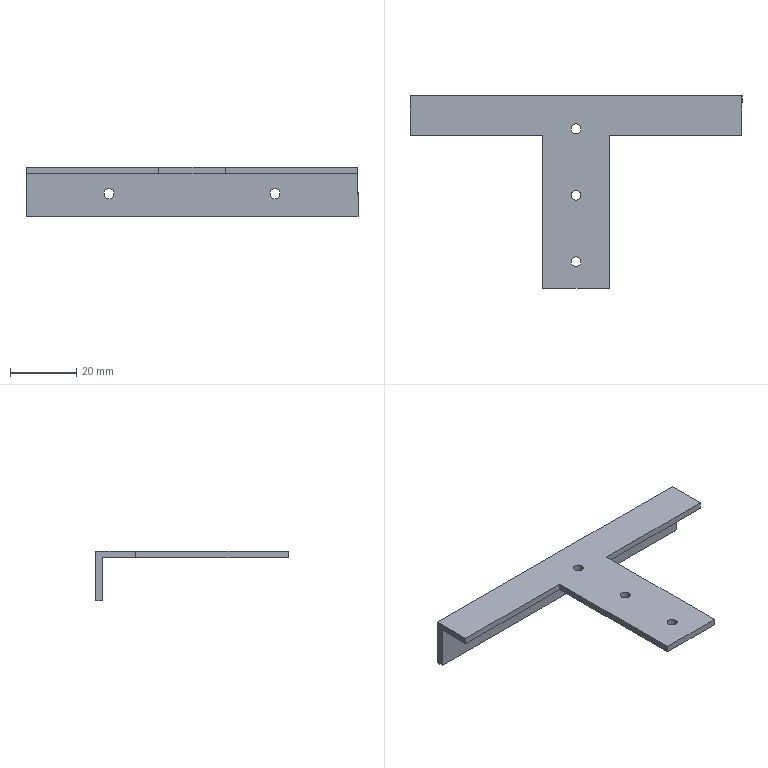Part | SolidWorks | features BaseBody 1 | 1 solid | 22 faces | box 100 x 58 x 15 mm | volume 6769 mm3 | plane 12 | cylinder 10 | commonest cylinder face diameters 3 x10
STEP:
#1=CARTESIAN_POINT('',(1.5,-30.,2.));
#2=VERTEX_POINT('',#1);
#3=CARTESIAN_POINT('',(-1.5,-30.,2.));
#4=VERTEX_POINT('',#3);
#5=CARTESIAN_POINT('',(0.,-30.,2.));
#6=DIRECTION('',(0.,0.,-1.));
#7=DIRECTION('',(-1.,0.,0.));
#8=AXIS2_PLACEMENT_3D('',#5,#6,#7);
#9=CIRCLE('',#8,1.5);
#10=EDGE_CURVE('',#2,#4,#9,.T.);
#11=ORIENTED_EDGE('',*,*,#10,.F.);
#12=CARTESIAN_POINT('',(1.5,-30.,0.));
#13=VERTEX_POINT('',#12);
#14=CARTESIAN_POINT('',(1.5,-30.,2.));
#15=DIRECTION('',(0.,0.,-1.));
#16=VECTOR('',#15,1000.);
#17=LINE('',#14,#16);
#18=EDGE_CURVE('',#2,#13,#17,.T.);
#19=ORIENTED_EDGE('',*,*,#18,.T.);
#20=CARTESIAN_POINT('',(-1.5,-30.,0.));
#21=VERTEX_POINT('',#20);
#22=CARTESIAN_POINT('',(0.,-30.,0.));
#23=DIRECTION('',(0.,0.,1.));
#24=DIRECTION('',(-1.,0.,0.));
#25=AXIS2_PLACEMENT_3D('',#22,#23,#24);
#26=CIRCLE('',#25,1.5);
#27=EDGE_CURVE('',#21,#13,#26,.T.);
#28=ORIENTED_EDGE('',*,*,#27,.F.);
#29=CARTESIAN_POINT('',(-1.5,-30.,2.));
#30=DIRECTION('',(0.,0.,-1.));
#31=VECTOR('',#30,1000.);
#32=LINE('',#29,#31);
#33=EDGE_CURVE('',#4,#21,#32,.T.);
#34=ORIENTED_EDGE('',*,*,#33,.F.);
#35=EDGE_LOOP('',(#11,#19,#28,#34));
#36=FACE_OUTER_BOUND('',#35,.T.);
#37=CARTESIAN_POINT('',(0.,-30.,2.));
#38=DIRECTION('',(0.,0.,-1.));
#39=DIRECTION('',(-1.,0.,0.));
#40=AXIS2_PLACEMENT_3D('',#37,#38,#39);
#41=CYLINDRICAL_SURFACE('',#40,1.5);
#42=ADVANCED_FACE('',(#36),#41,.F.);
#43=CARTESIAN_POINT('',(1.5,10.,2.));
#44=VERTEX_POINT('',#43);
#45=CARTESIAN_POINT('',(-1.5,10.,2.));
#46=VERTEX_POINT('',#45);
#47=CARTESIAN_POINT('',(0.,10.,2.));
#48=DIRECTION('',(0.,0.,-1.));
#49=DIRECTION('',(-1.,0.,0.));
#50=AXIS2_PLACEMENT_3D('',#47,#48,#49);
#51=CIRCLE('',#50,1.5);
#52=EDGE_CURVE('',#44,#46,#51,.T.);
#53=ORIENTED_EDGE('',*,*,#52,.F.);
#54=CARTESIAN_POINT('',(1.5,10.,0.));
#55=VERTEX_POINT('',#54);
#56=CARTESIAN_POINT('',(1.5,10.,2.));
#57=DIRECTION('',(0.,0.,-1.));
#58=VECTOR('',#57,1000.);
#59=LINE('',#56,#58);
#60=EDGE_CURVE('',#44,#55,#59,.T.);
#61=ORIENTED_EDGE('',*,*,#60,.T.);
#62=CARTESIAN_POINT('',(-1.5,10.,0.));
#63=VERTEX_POINT('',#62);
#64=CARTESIAN_POINT('',(0.,10.,0.));
#65=DIRECTION('',(0.,0.,1.));
#66=DIRECTION('',(-1.,0.,0.));
#67=AXIS2_PLACEMENT_3D('',#64,#65,#66);
#68=CIRCLE('',#67,1.5);
#69=EDGE_CURVE('',#63,#55,#68,.T.);
#70=ORIENTED_EDGE('',*,*,#69,.F.);
#71=CARTESIAN_POINT('',(-1.5,10.,2.));
#72=DIRECTION('',(0.,0.,-1.));
#73=VECTOR('',#72,1000.);
#74=LINE('',#71,#73);
#75=EDGE_CURVE('',#46,#63,#74,.T.);
#76=ORIENTED_EDGE('',*,*,#75,.F.);
#77=EDGE_LOOP('',(#53,#61,#70,#76));
#78=FACE_OUTER_BOUND('',#77,.T.);
#79=CARTESIAN_POINT('',(0.,10.,2.));
#80=DIRECTION('',(0.,0.,-1.));
#81=DIRECTION('',(-1.,0.,0.));
#82=AXIS2_PLACEMENT_3D('',#79,#80,#81);
#83=CYLINDRICAL_SURFACE('',#82,1.5);
#84=ADVANCED_FACE('',(#78),#83,.F.);
#85=CARTESIAN_POINT('',(1.5,-10.,2.));
#86=VERTEX_POINT('',#85);
#87=CARTESIAN_POINT('',(-1.5,-10.,2.));
#88=VERTEX_POINT('',#87);
#89=CARTESIAN_POINT('',(0.,-10.,2.));
#90=DIRECTION('',(0.,0.,-1.));
#91=DIRECTION('',(-1.,0.,0.));
#92=AXIS2_PLACEMENT_3D('',#89,#90,#91);
#93=CIRCLE('',#92,1.5);
#94=EDGE_CURVE('',#86,#88,#93,.T.);
#95=ORIENTED_EDGE('',*,*,#94,.F.);
#96=CARTESIAN_POINT('',(1.5,-10.,0.));
#97=VERTEX_POINT('',#96);
#98=CARTESIAN_POINT('',(1.5,-10.,2.));
#99=DIRECTION('',(0.,0.,-1.));
#100=VECTOR('',#99,1000.);
#101=LINE('',#98,#100);
#102=EDGE_CURVE('',#86,#97,#101,.T.);
#103=ORIENTED_EDGE('',*,*,#102,.T.);
#104=CARTESIAN_POINT('',(-1.5,-10.,0.));
#105=VERTEX_POINT('',#104);
#106=CARTESIAN_POINT('',(0.,-10.,0.));
#107=DIRECTION('',(0.,0.,1.));
#108=DIRECTION('',(-1.,0.,0.));
#109=AXIS2_PLACEMENT_3D('',#106,#107,#108);
#110=CIRCLE('',#109,1.5);
#111=EDGE_CURVE('',#105,#97,#110,.T.);
#112=ORIENTED_EDGE('',*,*,#111,.F.);
#113=CARTESIAN_POINT('',(-1.5,-10.,2.));
#114=DIRECTION('',(0.,0.,-1.));
#115=VECTOR('',#114,1000.);
#116=LINE('',#113,#115);
#117=EDGE_CURVE('',#88,#105,#116,.T.);
#118=ORIENTED_EDGE('',*,*,#117,.F.);
#119=EDGE_LOOP('',(#95,#103,#112,#118));
#120=FACE_OUTER_BOUND('',#119,.T.);
#121=CARTESIAN_POINT('',(0.,-10.,2.));
#122=DIRECTION('',(0.,0.,-1.));
#123=DIRECTION('',(-1.,0.,0.));
#124=AXIS2_PLACEMENT_3D('',#121,#122,#123);
#125=CYLINDRICAL_SURFACE('',#124,1.5);
#126=ADVANCED_FACE('',(#120),#125,.F.);
#127=CARTESIAN_POINT('',(25.,20.,-4.5));
#128=VERTEX_POINT('',#127);
#129=CARTESIAN_POINT('',(25.,20.,-7.5));
#130=VERTEX_POINT('',#129);
#131=CARTESIAN_POINT('',(25.,20.,-6.));
#132=DIRECTION('',(0.,-1.,0.));
#133=DIRECTION('',(0.,0.,-1.));
#134=AXIS2_PLACEMENT_3D('',#131,#132,#133);
#135=CIRCLE('',#134,1.5);
#136=EDGE_CURVE('',#128,#130,#135,.T.);
#137=ORIENTED_EDGE('',*,*,#136,.F.);
#138=CARTESIAN_POINT('',(25.,18.,-4.5));
#139=VERTEX_POINT('',#138);
#140=CARTESIAN_POINT('',(25.,28.,-4.5));
#141=DIRECTION('',(0.,-1.,0.));
#142=VECTOR('',#141,1000.);
#143=LINE('',#140,#142);
#144=EDGE_CURVE('',#128,#139,#143,.T.);
#145=ORIENTED_EDGE('',*,*,#144,.T.);
#146=CARTESIAN_POINT('',(25.,18.,-7.5));
#147=VERTEX_POINT('',#146);
#148=CARTESIAN_POINT('',(25.,18.,-6.));
#149=DIRECTION('',(0.,1.,0.));
#150=DIRECTION('',(0.,0.,-1.));
#151=AXIS2_PLACEMENT_3D('',#148,#149,#150);
#152=CIRCLE('',#151,1.5);
#153=EDGE_CURVE('',#147,#139,#152,.T.);
#154=ORIENTED_EDGE('',*,*,#153,.F.);
#155=CARTESIAN_POINT('',(25.,28.,-7.5));
#156=DIRECTION('',(0.,-1.,0.));
#157=VECTOR('',#156,1000.);
#158=LINE('',#155,#157);
#159=EDGE_CURVE('',#130,#147,#158,.T.);
#160=ORIENTED_EDGE('',*,*,#159,.F.);
#161=EDGE_LOOP('',(#137,#145,#154,#160));
#162=FACE_OUTER_BOUND('',#161,.T.);
#163=CARTESIAN_POINT('',(25.,28.,-6.));
#164=DIRECTION('',(0.,-1.,0.));
#165=DIRECTION('',(0.,0.,-1.));
#166=AXIS2_PLACEMENT_3D('',#163,#164,#165);
#167=CYLINDRICAL_SURFACE('',#166,1.5);
#168=ADVANCED_FACE('',(#162),#167,.F.);
#169=CARTESIAN_POINT('',(-25.,20.,-4.5));
#170=VERTEX_POINT('',#169);
#171=CARTESIAN_POINT('',(-25.,20.,-7.5));
#172=VERTEX_POINT('',#171);
#173=CARTESIAN_POINT('',(-25.,20.,-6.));
#174=DIRECTION('',(0.,-1.,0.));
#175=DIRECTION('',(0.,0.,-1.));
#176=AXIS2_PLACEMENT_3D('',#173,#174,#175);
#177=CIRCLE('',#176,1.5);
#178=EDGE_CURVE('',#170,#172,#177,.T.);
#179=ORIENTED_EDGE('',*,*,#178,.F.);
#180=CARTESIAN_POINT('',(-25.,18.,-4.5));
#181=VERTEX_POINT('',#180);
#182=CARTESIAN_POINT('',(-25.,28.,-4.5));
#183=DIRECTION('',(0.,-1.,0.));
#184=VECTOR('',#183,1000.);
#185=LINE('',#182,#184);
#186=EDGE_CURVE('',#170,#181,#185,.T.);
#187=ORIENTED_EDGE('',*,*,#186,.T.);
#188=CARTESIAN_POINT('',(-25.,18.,-7.5));
#189=VERTEX_POINT('',#188);
#190=CARTESIAN_POINT('',(-25.,18.,-6.));
#191=DIRECTION('',(0.,1.,0.));
#192=DIRECTION('',(0.,0.,-1.));
#193=AXIS2_PLACEMENT_3D('',#190,#191,#192);
#194=CIRCLE('',#193,1.5);
#195=EDGE_CURVE('',#189,#181,#194,.T.);
#196=ORIENTED_EDGE('',*,*,#195,.F.);
#197=CARTESIAN_POINT('',(-25.,28.,-7.5));
#198=DIRECTION('',(0.,-1.,0.));
#199=VECTOR('',#198,1000.);
#200=LINE('',#197,#199);
#201=EDGE_CURVE('',#172,#189,#200,.T.);
#202=ORIENTED_EDGE('',*,*,#201,.F.);
#203=EDGE_LOOP('',(#179,#187,#196,#202));
#204=FACE_OUTER_BOUND('',#203,.T.);
#205=CARTESIAN_POINT('',(-25.,28.,-6.));
#206=DIRECTION('',(0.,-1.,0.));
#207=DIRECTION('',(0.,0.,-1.));
#208=AXIS2_PLACEMENT_3D('',#205,#206,#207);
#209=CYLINDRICAL_SURFACE('',#208,1.5);
#210=ADVANCED_FACE('',(#204),#209,.F.);
#211=CARTESIAN_POINT('',(0.,-30.,2.));
#212=DIRECTION('',(0.,0.,-1.));
#213=DIRECTION('',(-1.,0.,0.));
#214=AXIS2_PLACEMENT_3D('',#211,#212,#213);
#215=CIRCLE('',#214,1.5);
#216=EDGE_CURVE('',#4,#2,#215,.T.);
#217=ORIENTED_EDGE('',*,*,#216,.T.);
#218=ORIENTED_EDGE('',*,*,#10,.T.);
#219=EDGE_LOOP('',(#217,#218));
#220=FACE_BOUND('',#219,.T.);
#221=CARTESIAN_POINT('',(0.,10.,2.));
#222=DIRECTION('',(0.,0.,-1.));
#223=DIRECTION('',(-1.,0.,0.));
#224=AXIS2_PLACEMENT_3D('',#221,#222,#223);
#225=CIRCLE('',#224,1.5);
#226=EDGE_CURVE('',#46,#44,#225,.T.);
#227=ORIENTED_EDGE('',*,*,#226,.T.);
#228=ORIENTED_EDGE('',*,*,#52,.T.);
#229=EDGE_LOOP('',(#227,#228));
#230=FACE_BOUND('',#229,.T.);
#231=CARTESIAN_POINT('',(50.,8.,2.));
#232=VERTEX_POINT('',#231);
#233=CARTESIAN_POINT('',(50.,20.,2.));
#234=VERTEX_POINT('',#233);
#235=CARTESIAN_POINT('',(50.,0.,2.));
#236=DIRECTION('',(0.,1.,0.));
#237=VECTOR('',#236,1000.);
#238=LINE('',#235,#237);
#239=EDGE_CURVE('',#232,#234,#238,.T.);
#240=ORIENTED_EDGE('',*,*,#239,.T.);
#241=CARTESIAN_POINT('',(-50.,20.,2.));
#242=VERTEX_POINT('',#241);
#243=CARTESIAN_POINT('',(0.,20.,2.));
#244=DIRECTION('',(-1.,0.,0.));
#245=VECTOR('',#244,1000.);
#246=LINE('',#243,#245);
#247=EDGE_CURVE('',#234,#242,#246,.T.);
#248=ORIENTED_EDGE('',*,*,#247,.T.);
#249=CARTESIAN_POINT('',(-50.,8.,2.));
#250=VERTEX_POINT('',#249);
#251=CARTESIAN_POINT('',(-50.,0.,2.));
#252=DIRECTION('',(0.,-1.,0.));
#253=VECTOR('',#252,1000.);
#254=LINE('',#251,#253);
#255=EDGE_CURVE('',#242,#250,#254,.T.);
#256=ORIENTED_EDGE('',*,*,#255,.T.);
#257=CARTESIAN_POINT('',(-10.,8.,2.));
#258=VERTEX_POINT('',#257);
#259=CARTESIAN_POINT('',(0.,8.,2.));
#260=DIRECTION('',(1.,0.,0.));
#261=VECTOR('',#260,1000.);
#262=LINE('',#259,#261);
#263=EDGE_CURVE('',#250,#258,#262,.T.);
#264=ORIENTED_EDGE('',*,*,#263,.T.);
#265=CARTESIAN_POINT('',(-10.,-38.,2.));
#266=VERTEX_POINT('',#265);
#267=CARTESIAN_POINT('',(-10.,0.,2.));
#268=DIRECTION('',(0.,-1.,0.));
#269=VECTOR('',#268,1000.);
#270=LINE('',#267,#269);
#271=EDGE_CURVE('',#258,#266,#270,.T.);
#272=ORIENTED_EDGE('',*,*,#271,.T.);
#273=CARTESIAN_POINT('',(10.,-38.,2.));
#274=VERTEX_POINT('',#273);
#275=CARTESIAN_POINT('',(0.,-38.,2.));
#276=DIRECTION('',(1.,0.,0.));
#277=VECTOR('',#276,1000.);
#278=LINE('',#275,#277);
#279=EDGE_CURVE('',#266,#274,#278,.T.);
#280=ORIENTED_EDGE('',*,*,#279,.T.);
#281=CARTESIAN_POINT('',(10.,8.,2.));
#282=VERTEX_POINT('',#281);
#283=CARTESIAN_POINT('',(10.,0.,2.));
#284=DIRECTION('',(0.,1.,0.));
#285=VECTOR('',#284,1000.);
#286=LINE('',#283,#285);
#287=EDGE_CURVE('',#274,#282,#286,.T.);
#288=ORIENTED_EDGE('',*,*,#287,.T.);
#289=CARTESIAN_POINT('',(0.,8.,2.));
#290=DIRECTION('',(1.,0.,0.));
#291=VECTOR('',#290,1000.);
#292=LINE('',#289,#291);
#293=EDGE_CURVE('',#282,#232,#292,.T.);
#294=ORIENTED_EDGE('',*,*,#293,.T.);
#295=EDGE_LOOP('',(#240,#248,#256,#264,#272,#280,#288,#294));
#296=FACE_OUTER_BOUND('',#295,.T.);
#297=CARTESIAN_POINT('',(0.,-10.,2.));
#298=DIRECTION('',(0.,0.,-1.));
#299=DIRECTION('',(-1.,0.,0.));
#300=AXIS2_PLACEMENT_3D('',#297,#298,#299);
#301=CIRCLE('',#300,1.5);
#302=EDGE_CURVE('',#88,#86,#301,.T.);
#303=ORIENTED_EDGE('',*,*,#302,.T.);
#304=ORIENTED_EDGE('',*,*,#94,.T.);
#305=EDGE_LOOP('',(#303,#304));
#306=FACE_BOUND('',#305,.T.);
#307=CARTESIAN_POINT('',(0.,0.,2.));
#308=DIRECTION('',(0.,0.,1.));
#309=DIRECTION('',(1.,0.,0.));
#310=AXIS2_PLACEMENT_3D('',#307,#308,#309);
#311=PLANE('',#310);
#312=ADVANCED_FACE('',(#220,#230,#296,#306),#311,.T.);
#313=ORIENTED_EDGE('',*,*,#18,.F.);
#314=ORIENTED_EDGE('',*,*,#216,.F.);
#315=ORIENTED_EDGE('',*,*,#33,.T.);
#316=CARTESIAN_POINT('',(0.,-30.,0.));
#317=DIRECTION('',(0.,0.,1.));
#318=DIRECTION('',(-1.,0.,0.));
#319=AXIS2_PLACEMENT_3D('',#316,#317,#318);
#320=CIRCLE('',#319,1.5);
#321=EDGE_CURVE('',#13,#21,#320,.T.);
#322=ORIENTED_EDGE('',*,*,#321,.F.);
#323=EDGE_LOOP('',(#313,#314,#315,#322));
#324=FACE_OUTER_BOUND('',#323,.T.);
#325=CARTESIAN_POINT('',(0.,-30.,2.));
#326=DIRECTION('',(0.,0.,-1.));
#327=DIRECTION('',(-1.,0.,0.));
#328=AXIS2_PLACEMENT_3D('',#325,#326,#327);
#329=CYLINDRICAL_SURFACE('',#328,1.5);
#330=ADVANCED_FACE('',(#324),#329,.F.);
#331=ORIENTED_EDGE('',*,*,#60,.F.);
#332=ORIENTED_EDGE('',*,*,#226,.F.);
#333=ORIENTED_EDGE('',*,*,#75,.T.);
#334=CARTESIAN_POINT('',(0.,10.,0.));
#335=DIRECTION('',(0.,0.,1.));
#336=DIRECTION('',(-1.,0.,0.));
#337=AXIS2_PLACEMENT_3D('',#334,#335,#336);
#338=CIRCLE('',#337,1.5);
#339=EDGE_CURVE('',#55,#63,#338,.T.);
#340=ORIENTED_EDGE('',*,*,#339,.F.);
#341=EDGE_LOOP('',(#331,#332,#333,#340));
#342=FACE_OUTER_BOUND('',#341,.T.);
#343=CARTESIAN_POINT('',(0.,10.,2.));
#344=DIRECTION('',(0.,0.,-1.));
#345=DIRECTION('',(-1.,0.,0.));
#346=AXIS2_PLACEMENT_3D('',#343,#344,#345);
#347=CYLINDRICAL_SURFACE('',#346,1.5);
#348=ADVANCED_FACE('',(#342),#347,.F.);
#349=CARTESIAN_POINT('',(25.,20.,-6.));
#350=DIRECTION('',(0.,-1.,0.));
#351=DIRECTION('',(0.,0.,-1.));
#352=AXIS2_PLACEMENT_3D('',#349,#350,#351);
#353=CIRCLE('',#352,1.5);
#354=EDGE_CURVE('',#130,#128,#353,.T.);
#355=ORIENTED_EDGE('',*,*,#354,.T.);
#356=ORIENTED_EDGE('',*,*,#136,.T.);
#357=EDGE_LOOP('',(#355,#356));
#358=FACE_BOUND('',#357,.T.);
#359=CARTESIAN_POINT('',(-25.,20.,-6.));
#360=DIRECTION('',(0.,-1.,0.));
#361=DIRECTION('',(0.,0.,-1.));
#362=AXIS2_PLACEMENT_3D('',#359,#360,#361);
#363=CIRCLE('',#362,1.5);
#364=EDGE_CURVE('',#172,#170,#363,.T.);
#365=ORIENTED_EDGE('',*,*,#364,.T.);
#366=ORIENTED_EDGE('',*,*,#178,.T.);
#367=EDGE_LOOP('',(#365,#366));
#368=FACE_BOUND('',#367,.T.);
#369=CARTESIAN_POINT('',(50.,20.,-13.));
#370=VERTEX_POINT('',#369);
#371=CARTESIAN_POINT('',(50.,20.,0.));
#372=DIRECTION('',(0.,0.,-1.));
#373=VECTOR('',#372,1000.);
#374=LINE('',#371,#373);
#375=EDGE_CURVE('',#234,#370,#374,.T.);
#376=ORIENTED_EDGE('',*,*,#375,.T.);
#377=CARTESIAN_POINT('',(-50.,20.,-13.));
#378=VERTEX_POINT('',#377);
#379=CARTESIAN_POINT('',(0.,20.,-13.));
#380=DIRECTION('',(-1.,0.,0.));
#381=VECTOR('',#380,1000.);
#382=LINE('',#379,#381);
#383=EDGE_CURVE('',#370,#378,#382,.T.);
#384=ORIENTED_EDGE('',*,*,#383,.T.);
#385=CARTESIAN_POINT('',(-50.,20.,0.));
#386=DIRECTION('',(0.,0.,1.));
#387=VECTOR('',#386,1000.);
#388=LINE('',#385,#387);
#389=EDGE_CURVE('',#378,#242,#388,.T.);
#390=ORIENTED_EDGE('',*,*,#389,.T.);
#391=ORIENTED_EDGE('',*,*,#247,.F.);
#392=EDGE_LOOP('',(#376,#384,#390,#391));
#393=FACE_OUTER_BOUND('',#392,.T.);
#394=CARTESIAN_POINT('',(0.,20.,0.));
#395=DIRECTION('',(0.,1.,0.));
#396=DIRECTION('',(0.,0.,1.));
#397=AXIS2_PLACEMENT_3D('',#394,#395,#396);
#398=PLANE('',#397);
#399=ADVANCED_FACE('',(#358,#368,#393),#398,.T.);
#400=CARTESIAN_POINT('',(50.,18.,-13.));
#401=VERTEX_POINT('',#400);
#402=CARTESIAN_POINT('',(50.,18.,0.));
#403=VERTEX_POINT('',#402);
#404=CARTESIAN_POINT('',(50.,18.,2.));
#405=DIRECTION('',(0.,0.,1.));
#406=VECTOR('',#405,1000.);
#407=LINE('',#404,#406);
#408=EDGE_CURVE('',#401,#403,#407,.T.);
#409=ORIENTED_EDGE('',*,*,#408,.F.);
#410=CARTESIAN_POINT('',(50.,18.,-13.));
#411=DIRECTION('',(0.,-1.,0.));
#412=VECTOR('',#411,1000.);
#413=LINE('',#410,#412);
#414=EDGE_CURVE('',#370,#401,#413,.T.);
#415=ORIENTED_EDGE('',*,*,#414,.F.);
#416=ORIENTED_EDGE('',*,*,#375,.F.);
#417=ORIENTED_EDGE('',*,*,#239,.F.);
#418=CARTESIAN_POINT('',(50.,8.,0.));
#419=VERTEX_POINT('',#418);
#420=CARTESIAN_POINT('',(50.,8.,2.));
#421=DIRECTION('',(0.,0.,1.));
#422=VECTOR('',#421,1000.);
#423=LINE('',#420,#422);
#424=EDGE_CURVE('',#419,#232,#423,.T.);
#425=ORIENTED_EDGE('',*,*,#424,.F.);
#426=CARTESIAN_POINT('',(50.,18.,0.));
#427=DIRECTION('',(0.,-1.,0.));
#428=VECTOR('',#427,1000.);
#429=LINE('',#426,#428);
#430=EDGE_CURVE('',#403,#419,#429,.T.);
#431=ORIENTED_EDGE('',*,*,#430,.F.);
#432=EDGE_LOOP('',(#409,#415,#416,#417,#425,#431));
#433=FACE_OUTER_BOUND('',#432,.T.);
#434=CARTESIAN_POINT('',(50.,18.,2.));
#435=DIRECTION('',(-1.,0.,0.));
#436=DIRECTION('',(0.,-1.,0.));
#437=AXIS2_PLACEMENT_3D('',#434,#435,#436);
#438=PLANE('',#437);
#439=ADVANCED_FACE('',(#433),#438,.F.);
#440=ORIENTED_EDGE('',*,*,#424,.T.);
#441=ORIENTED_EDGE('',*,*,#293,.F.);
#442=CARTESIAN_POINT('',(10.,8.,0.));
#443=VERTEX_POINT('',#442);
#444=CARTESIAN_POINT('',(10.,8.,2.));
#445=DIRECTION('',(0.,0.,1.));
#446=VECTOR('',#445,1000.);
#447=LINE('',#444,#446);
#448=EDGE_CURVE('',#443,#282,#447,.T.);
#449=ORIENTED_EDGE('',*,*,#448,.F.);
#450=CARTESIAN_POINT('',(50.,8.,0.));
#451=DIRECTION('',(-1.,0.,0.));
#452=VECTOR('',#451,1000.);
#453=LINE('',#450,#452);
#454=EDGE_CURVE('',#419,#443,#453,.T.);
#455=ORIENTED_EDGE('',*,*,#454,.F.);
#456=EDGE_LOOP('',(#440,#441,#449,#455));
#457=FACE_OUTER_BOUND('',#456,.T.);
#458=CARTESIAN_POINT('',(50.,8.,2.));
#459=DIRECTION('',(0.,1.,0.));
#460=DIRECTION('',(-1.,0.,0.));
#461=AXIS2_PLACEMENT_3D('',#458,#459,#460);
#462=PLANE('',#461);
#463=ADVANCED_FACE('',(#457),#462,.F.);
#464=ORIENTED_EDGE('',*,*,#448,.T.);
#465=ORIENTED_EDGE('',*,*,#287,.F.);
#466=CARTESIAN_POINT('',(10.,-38.,0.));
#467=VERTEX_POINT('',#466);
#468=CARTESIAN_POINT('',(10.,-38.,2.));
#469=DIRECTION('',(0.,0.,1.));
#470=VECTOR('',#469,1000.);
#471=LINE('',#468,#470);
#472=EDGE_CURVE('',#467,#274,#471,.T.);
#473=ORIENTED_EDGE('',*,*,#472,.F.);
#474=CARTESIAN_POINT('',(10.,8.,0.));
#475=DIRECTION('',(0.,-1.,0.));
#476=VECTOR('',#475,1000.);
#477=LINE('',#474,#476);
#478=EDGE_CURVE('',#443,#467,#477,.T.);
#479=ORIENTED_EDGE('',*,*,#478,.F.);
#480=EDGE_LOOP('',(#464,#465,#473,#479));
#481=FACE_OUTER_BOUND('',#480,.T.);
#482=CARTESIAN_POINT('',(10.,8.,2.));
#483=DIRECTION('',(-1.,0.,0.));
#484=DIRECTION('',(0.,-1.,0.));
#485=AXIS2_PLACEMENT_3D('',#482,#483,#484);
#486=PLANE('',#485);
#487=ADVANCED_FACE('',(#481),#486,.F.);
#488=ORIENTED_EDGE('',*,*,#472,.T.);
#489=ORIENTED_EDGE('',*,*,#279,.F.);
#490=CARTESIAN_POINT('',(-10.,-38.,0.));
#491=VERTEX_POINT('',#490);
#492=CARTESIAN_POINT('',(-10.,-38.,2.));
#493=DIRECTION('',(0.,0.,1.));
#494=VECTOR('',#493,1000.);
#495=LINE('',#492,#494);
#496=EDGE_CURVE('',#491,#266,#495,.T.);
#497=ORIENTED_EDGE('',*,*,#496,.F.);
#498=CARTESIAN_POINT('',(-10.,-38.,0.));
#499=DIRECTION('',(-1.,0.,0.));
#500=VECTOR('',#499,1000.);
#501=LINE('',#498,#500);
#502=EDGE_CURVE('',#467,#491,#501,.T.);
#503=ORIENTED_EDGE('',*,*,#502,.F.);
#504=EDGE_LOOP('',(#488,#489,#497,#503));
#505=FACE_OUTER_BOUND('',#504,.T.);
#506=CARTESIAN_POINT('',(-10.,-38.,2.));
#507=DIRECTION('',(0.,1.,0.));
#508=DIRECTION('',(0.,0.,1.));
#509=AXIS2_PLACEMENT_3D('',#506,#507,#508);
#510=PLANE('',#509);
#511=ADVANCED_FACE('',(#505),#510,.F.);
#512=ORIENTED_EDGE('',*,*,#496,.T.);
#513=ORIENTED_EDGE('',*,*,#271,.F.);
#514=CARTESIAN_POINT('',(-10.,8.,0.));
#515=VERTEX_POINT('',#514);
#516=CARTESIAN_POINT('',(-10.,8.,2.));
#517=DIRECTION('',(0.,0.,1.));
#518=VECTOR('',#517,1000.);
#519=LINE('',#516,#518);
#520=EDGE_CURVE('',#515,#258,#519,.T.);
#521=ORIENTED_EDGE('',*,*,#520,.F.);
#522=CARTESIAN_POINT('',(-10.,8.,0.));
#523=DIRECTION('',(0.,1.,0.));
#524=VECTOR('',#523,1000.);
#525=LINE('',#522,#524);
#526=EDGE_CURVE('',#491,#515,#525,.T.);
#527=ORIENTED_EDGE('',*,*,#526,.F.);
#528=EDGE_LOOP('',(#512,#513,#521,#527));
#529=FACE_OUTER_BOUND('',#528,.T.);
#530=CARTESIAN_POINT('',(-10.,8.,2.));
#531=DIRECTION('',(1.,0.,0.));
#532=DIRECTION('',(0.,1.,0.));
#533=AXIS2_PLACEMENT_3D('',#530,#531,#532);
#534=PLANE('',#533);
#535=ADVANCED_FACE('',(#529),#534,.F.);
#536=ORIENTED_EDGE('',*,*,#520,.T.);
#537=ORIENTED_EDGE('',*,*,#263,.F.);
#538=CARTESIAN_POINT('',(-50.,8.,0.));
#539=VERTEX_POINT('',#538);
#540=CARTESIAN_POINT('',(-50.,8.,2.));
#541=DIRECTION('',(0.,0.,1.));
#542=VECTOR('',#541,1000.);
#543=LINE('',#540,#542);
#544=EDGE_CURVE('',#539,#250,#543,.T.);
#545=ORIENTED_EDGE('',*,*,#544,.F.);
#546=CARTESIAN_POINT('',(-50.,8.,0.));
#547=DIRECTION('',(-1.,0.,0.));
#548=VECTOR('',#547,1000.);
#549=LINE('',#546,#548);
#550=EDGE_CURVE('',#515,#539,#549,.T.);
#551=ORIENTED_EDGE('',*,*,#550,.F.);
#552=EDGE_LOOP('',(#536,#537,#545,#551));
#553=FACE_OUTER_BOUND('',#552,.T.);
#554=CARTESIAN_POINT('',(-50.,8.,2.));
#555=DIRECTION('',(0.,1.,0.));
#556=DIRECTION('',(0.,0.,1.));
#557=AXIS2_PLACEMENT_3D('',#554,#555,#556);
#558=PLANE('',#557);
#559=ADVANCED_FACE('',(#553),#558,.F.);
#560=ORIENTED_EDGE('',*,*,#544,.T.);
#561=ORIENTED_EDGE('',*,*,#255,.F.);
#562=ORIENTED_EDGE('',*,*,#389,.F.);
#563=CARTESIAN_POINT('',(-50.,18.,-13.));
#564=VERTEX_POINT('',#563);
#565=CARTESIAN_POINT('',(-50.,18.,-13.));
#566=DIRECTION('',(0.,1.,0.));
#567=VECTOR('',#566,1000.);
#568=LINE('',#565,#567);
#569=EDGE_CURVE('',#564,#378,#568,.T.);
#570=ORIENTED_EDGE('',*,*,#569,.F.);
#571=CARTESIAN_POINT('',(-50.,18.,0.));
#572=VERTEX_POINT('',#571);
#573=CARTESIAN_POINT('',(-50.,18.,2.));
#574=DIRECTION('',(0.,0.,-1.));
#575=VECTOR('',#574,1000.);
#576=LINE('',#573,#575);
#577=EDGE_CURVE('',#572,#564,#576,.T.);
#578=ORIENTED_EDGE('',*,*,#577,.F.);
#579=CARTESIAN_POINT('',(-50.,18.,0.));
#580=DIRECTION('',(0.,1.,0.));
#581=VECTOR('',#580,1000.);
#582=LINE('',#579,#581);
#583=EDGE_CURVE('',#539,#572,#582,.T.);
#584=ORIENTED_EDGE('',*,*,#583,.F.);
#585=EDGE_LOOP('',(#560,#561,#562,#570,#578,#584));
#586=FACE_OUTER_BOUND('',#585,.T.);
#587=CARTESIAN_POINT('',(-50.,18.,2.));
#588=DIRECTION('',(1.,0.,0.));
#589=DIRECTION('',(0.,1.,0.));
#590=AXIS2_PLACEMENT_3D('',#587,#588,#589);
#591=PLANE('',#590);
#592=ADVANCED_FACE('',(#586),#591,.F.);
#593=ORIENTED_EDGE('',*,*,#102,.F.);
#594=ORIENTED_EDGE('',*,*,#302,.F.);
#595=ORIENTED_EDGE('',*,*,#117,.T.);
#596=CARTESIAN_POINT('',(0.,-10.,0.));
#597=DIRECTION('',(0.,0.,1.));
#598=DIRECTION('',(-1.,0.,0.));
#599=AXIS2_PLACEMENT_3D('',#596,#597,#598);
#600=CIRCLE('',#599,1.5);
#601=EDGE_CURVE('',#97,#105,#600,.T.);
#602=ORIENTED_EDGE('',*,*,#601,.F.);
#603=EDGE_LOOP('',(#593,#594,#595,#602));
#604=FACE_OUTER_BOUND('',#603,.T.);
#605=CARTESIAN_POINT('',(0.,-10.,2.));
#606=DIRECTION('',(0.,0.,-1.));
#607=DIRECTION('',(-1.,0.,0.));
#608=AXIS2_PLACEMENT_3D('',#605,#606,#607);
#609=CYLINDRICAL_SURFACE('',#608,1.5);
#610=ADVANCED_FACE('',(#604),#609,.F.);
#611=ORIENTED_EDGE('',*,*,#27,.T.);
#612=ORIENTED_EDGE('',*,*,#321,.T.);
#613=EDGE_LOOP('',(#611,#612));
#614=FACE_BOUND('',#613,.T.);
#615=ORIENTED_EDGE('',*,*,#111,.T.);
#616=ORIENTED_EDGE('',*,*,#601,.T.);
#617=EDGE_LOOP('',(#615,#616));
#618=FACE_BOUND('',#617,.T.);
#619=ORIENTED_EDGE('',*,*,#69,.T.);
#620=ORIENTED_EDGE('',*,*,#339,.T.);
#621=EDGE_LOOP('',(#619,#620));
#622=FACE_BOUND('',#621,.T.);
#623=CARTESIAN_POINT('',(0.,18.,0.));
#624=DIRECTION('',(-1.,0.,0.));
#625=VECTOR('',#624,1000.);
#626=LINE('',#623,#625);
#627=EDGE_CURVE('',#403,#572,#626,.T.);
#628=ORIENTED_EDGE('',*,*,#627,.F.);
#629=ORIENTED_EDGE('',*,*,#430,.T.);
#630=ORIENTED_EDGE('',*,*,#454,.T.);
#631=ORIENTED_EDGE('',*,*,#478,.T.);
#632=ORIENTED_EDGE('',*,*,#502,.T.);
#633=ORIENTED_EDGE('',*,*,#526,.T.);
#634=ORIENTED_EDGE('',*,*,#550,.T.);
#635=ORIENTED_EDGE('',*,*,#583,.T.);
#636=EDGE_LOOP('',(#628,#629,#630,#631,#632,#633,#634,#635));
#637=FACE_OUTER_BOUND('',#636,.T.);
#638=CARTESIAN_POINT('',(0.,0.,0.));
#639=DIRECTION('',(0.,0.,1.));
#640=DIRECTION('',(1.,0.,0.));
#641=AXIS2_PLACEMENT_3D('',#638,#639,#640);
#642=PLANE('',#641);
#643=ADVANCED_FACE('',(#614,#618,#622,#637),#642,.F.);
#644=ORIENTED_EDGE('',*,*,#144,.F.);
#645=ORIENTED_EDGE('',*,*,#354,.F.);
#646=ORIENTED_EDGE('',*,*,#159,.T.);
#647=CARTESIAN_POINT('',(25.,18.,-6.));
#648=DIRECTION('',(0.,1.,0.));
#649=DIRECTION('',(0.,0.,-1.));
#650=AXIS2_PLACEMENT_3D('',#647,#648,#649);
#651=CIRCLE('',#650,1.5);
#652=EDGE_CURVE('',#139,#147,#651,.T.);
#653=ORIENTED_EDGE('',*,*,#652,.F.);
#654=EDGE_LOOP('',(#644,#645,#646,#653));
#655=FACE_OUTER_BOUND('',#654,.T.);
#656=CARTESIAN_POINT('',(25.,28.,-6.));
#657=DIRECTION('',(0.,-1.,0.));
#658=DIRECTION('',(0.,0.,-1.));
#659=AXIS2_PLACEMENT_3D('',#656,#657,#658);
#660=CYLINDRICAL_SURFACE('',#659,1.5);
#661=ADVANCED_FACE('',(#655),#660,.F.);
#662=ORIENTED_EDGE('',*,*,#186,.F.);
#663=ORIENTED_EDGE('',*,*,#364,.F.);
#664=ORIENTED_EDGE('',*,*,#201,.T.);
#665=CARTESIAN_POINT('',(-25.,18.,-6.));
#666=DIRECTION('',(0.,1.,0.));
#667=DIRECTION('',(0.,0.,-1.));
#668=AXIS2_PLACEMENT_3D('',#665,#666,#667);
#669=CIRCLE('',#668,1.5);
#670=EDGE_CURVE('',#181,#189,#669,.T.);
#671=ORIENTED_EDGE('',*,*,#670,.F.);
#672=EDGE_LOOP('',(#662,#663,#664,#671));
#673=FACE_OUTER_BOUND('',#672,.T.);
#674=CARTESIAN_POINT('',(-25.,28.,-6.));
#675=DIRECTION('',(0.,-1.,0.));
#676=DIRECTION('',(0.,0.,-1.));
#677=AXIS2_PLACEMENT_3D('',#674,#675,#676);
#678=CYLINDRICAL_SURFACE('',#677,1.5);
#679=ADVANCED_FACE('',(#673),#678,.F.);
#680=ORIENTED_EDGE('',*,*,#569,.T.);
#681=ORIENTED_EDGE('',*,*,#383,.F.);
#682=ORIENTED_EDGE('',*,*,#414,.T.);
#683=CARTESIAN_POINT('',(50.,18.,-13.));
#684=DIRECTION('',(1.,0.,0.));
#685=VECTOR('',#684,1000.);
#686=LINE('',#683,#685);
#687=EDGE_CURVE('',#564,#401,#686,.T.);
#688=ORIENTED_EDGE('',*,*,#687,.F.);
#689=EDGE_LOOP('',(#680,#681,#682,#688));
#690=FACE_OUTER_BOUND('',#689,.T.);
#691=CARTESIAN_POINT('',(50.,20.,-13.));
#692=DIRECTION('',(0.,0.,1.));
#693=DIRECTION('',(1.,0.,0.));
#694=AXIS2_PLACEMENT_3D('',#691,#692,#693);
#695=PLANE('',#694);
#696=ADVANCED_FACE('',(#690),#695,.F.);
#697=ORIENTED_EDGE('',*,*,#153,.T.);
#698=ORIENTED_EDGE('',*,*,#652,.T.);
#699=EDGE_LOOP('',(#697,#698));
#700=FACE_BOUND('',#699,.T.);
#701=ORIENTED_EDGE('',*,*,#627,.T.);
#702=ORIENTED_EDGE('',*,*,#577,.T.);
#703=ORIENTED_EDGE('',*,*,#687,.T.);
#704=ORIENTED_EDGE('',*,*,#408,.T.);
#705=EDGE_LOOP('',(#701,#702,#703,#704));
#706=FACE_OUTER_BOUND('',#705,.T.);
#707=ORIENTED_EDGE('',*,*,#195,.T.);
#708=ORIENTED_EDGE('',*,*,#670,.T.);
#709=EDGE_LOOP('',(#707,#708));
#710=FACE_BOUND('',#709,.T.);
#711=CARTESIAN_POINT('',(0.,18.,0.));
#712=DIRECTION('',(0.,1.,0.));
#713=DIRECTION('',(0.,0.,1.));
#714=AXIS2_PLACEMENT_3D('',#711,#712,#713);
#715=PLANE('',#714);
#716=ADVANCED_FACE('',(#700,#706,#710),#715,.F.);
#717=CLOSED_SHELL('',(#42,#84,#126,#168,#210,#312,#330,#348,#399,#439,#463,#487,#511,#535,#559,#592,#610,#643,#661,#679,#696,#716));
#718=MANIFOLD_SOLID_BREP('',#717);
#719=CARTESIAN_POINT('',(0.,0.,0.));
#720=DIRECTION('',(0.,0.,1.));
#721=DIRECTION('',(1.,0.,0.));
#722=AXIS2_PLACEMENT_3D('',#719,#720,#721);
#723=(LENGTH_UNIT()NAMED_UNIT(*)SI_UNIT(.MILLI.,.METRE.));
#724=UNCERTAINTY_MEASURE_WITH_UNIT(LENGTH_MEASURE(0.00001),#723,'','');
#725=(NAMED_UNIT(*)PLANE_ANGLE_UNIT()SI_UNIT($,.RADIAN.));
#726=(NAMED_UNIT(*)SI_UNIT($,.STERADIAN.)SOLID_ANGLE_UNIT());
#727=(GEOMETRIC_REPRESENTATION_CONTEXT(3)GLOBAL_UNCERTAINTY_ASSIGNED_CONTEXT((#724))GLOBAL_UNIT_ASSIGNED_CONTEXT((#723,#725,#726))REPRESENTATION_CONTEXT('',''));
#728=ADVANCED_BREP_SHAPE_REPRESENTATION('',(#718,#722),#727);